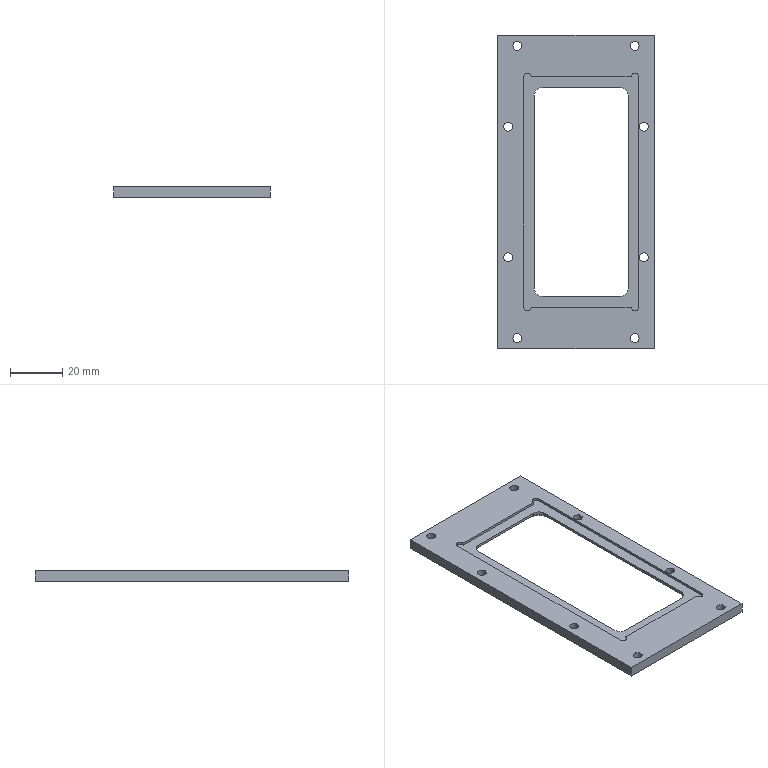Part | 1 solid | 63 faces | box 60 x 120 x 4 mm | volume 15362 mm3 | cylinder 24 | cone 20 | plane 19 | commonest cylinder face diameters 3.4 x16 3 x4 6 x4